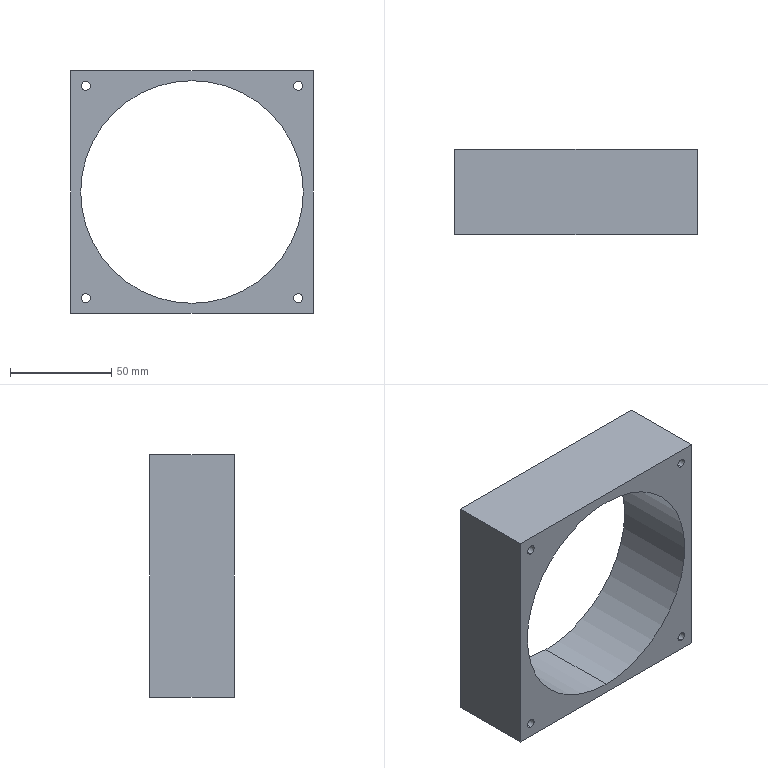Part | SolidWorks | features Extrusion 1, ICE 1 | 1 solid | 16 faces | box 120 x 42 x 120 mm | volume 202989 mm3 | cylinder 10 | plane 6 | commonest cylinder face diameters 4.5 x8 110 x2
STEP:
#1=CARTESIAN_POINT('',(-52.5,-21.,50.25));
#2=VERTEX_POINT('',#1);
#3=CARTESIAN_POINT('',(-52.5,-21.,54.75));
#4=VERTEX_POINT('',#3);
#5=CARTESIAN_POINT('',(-52.5,-21.,52.5));
#6=DIRECTION('',(0.,1.,0.));
#7=DIRECTION('',(0.,0.,-1.));
#8=AXIS2_PLACEMENT_3D('',#5,#6,#7);
#9=CIRCLE('',#8,2.25);
#10=EDGE_CURVE('',#2,#4,#9,.T.);
#11=ORIENTED_EDGE('',*,*,#10,.F.);
#12=CARTESIAN_POINT('',(-52.5,21.,50.25));
#13=VERTEX_POINT('',#12);
#14=CARTESIAN_POINT('',(-52.5,-21.,50.25));
#15=DIRECTION('',(0.,1.,0.));
#16=VECTOR('',#15,1000.);
#17=LINE('',#14,#16);
#18=EDGE_CURVE('',#2,#13,#17,.T.);
#19=ORIENTED_EDGE('',*,*,#18,.T.);
#20=CARTESIAN_POINT('',(-52.5,21.,54.75));
#21=VERTEX_POINT('',#20);
#22=CARTESIAN_POINT('',(-52.5,21.,52.5));
#23=DIRECTION('',(0.,1.,0.));
#24=DIRECTION('',(0.,0.,1.));
#25=AXIS2_PLACEMENT_3D('',#22,#23,#24);
#26=CIRCLE('',#25,2.25);
#27=EDGE_CURVE('',#13,#21,#26,.T.);
#28=ORIENTED_EDGE('',*,*,#27,.T.);
#29=CARTESIAN_POINT('',(-52.5,-21.,54.75));
#30=DIRECTION('',(0.,1.,0.));
#31=VECTOR('',#30,1000.);
#32=LINE('',#29,#31);
#33=EDGE_CURVE('',#4,#21,#32,.T.);
#34=ORIENTED_EDGE('',*,*,#33,.F.);
#35=EDGE_LOOP('',(#11,#19,#28,#34));
#36=FACE_OUTER_BOUND('',#35,.T.);
#37=CARTESIAN_POINT('',(-52.5,-21.,52.5));
#38=DIRECTION('',(0.,1.,0.));
#39=DIRECTION('',(0.,0.,1.));
#40=AXIS2_PLACEMENT_3D('',#37,#38,#39);
#41=CYLINDRICAL_SURFACE('',#40,2.25);
#42=ADVANCED_FACE('',(#36),#41,.F.);
#43=CARTESIAN_POINT('',(52.5,-21.,50.25));
#44=VERTEX_POINT('',#43);
#45=CARTESIAN_POINT('',(52.5,-21.,54.75));
#46=VERTEX_POINT('',#45);
#47=CARTESIAN_POINT('',(52.5,-21.,52.5));
#48=DIRECTION('',(0.,1.,0.));
#49=DIRECTION('',(0.,0.,1.));
#50=AXIS2_PLACEMENT_3D('',#47,#48,#49);
#51=CIRCLE('',#50,2.25);
#52=EDGE_CURVE('',#44,#46,#51,.T.);
#53=ORIENTED_EDGE('',*,*,#52,.F.);
#54=CARTESIAN_POINT('',(52.5,21.,50.25));
#55=VERTEX_POINT('',#54);
#56=CARTESIAN_POINT('',(52.5,-21.,50.25));
#57=DIRECTION('',(0.,1.,0.));
#58=VECTOR('',#57,1000.);
#59=LINE('',#56,#58);
#60=EDGE_CURVE('',#44,#55,#59,.T.);
#61=ORIENTED_EDGE('',*,*,#60,.T.);
#62=CARTESIAN_POINT('',(52.5,21.,54.75));
#63=VERTEX_POINT('',#62);
#64=CARTESIAN_POINT('',(52.5,21.,52.5));
#65=DIRECTION('',(0.,1.,0.));
#66=DIRECTION('',(0.,0.,1.));
#67=AXIS2_PLACEMENT_3D('',#64,#65,#66);
#68=CIRCLE('',#67,2.25);
#69=EDGE_CURVE('',#55,#63,#68,.T.);
#70=ORIENTED_EDGE('',*,*,#69,.T.);
#71=CARTESIAN_POINT('',(52.5,-21.,54.75));
#72=DIRECTION('',(0.,1.,0.));
#73=VECTOR('',#72,1000.);
#74=LINE('',#71,#73);
#75=EDGE_CURVE('',#46,#63,#74,.T.);
#76=ORIENTED_EDGE('',*,*,#75,.F.);
#77=EDGE_LOOP('',(#53,#61,#70,#76));
#78=FACE_OUTER_BOUND('',#77,.T.);
#79=CARTESIAN_POINT('',(52.5,-21.,52.5));
#80=DIRECTION('',(0.,1.,0.));
#81=DIRECTION('',(0.,0.,1.));
#82=AXIS2_PLACEMENT_3D('',#79,#80,#81);
#83=CYLINDRICAL_SURFACE('',#82,2.25);
#84=ADVANCED_FACE('',(#78),#83,.F.);
#85=CARTESIAN_POINT('',(52.5,-21.,-54.75));
#86=VERTEX_POINT('',#85);
#87=CARTESIAN_POINT('',(52.5,-21.,-50.25));
#88=VERTEX_POINT('',#87);
#89=CARTESIAN_POINT('',(52.5,-21.,-52.5));
#90=DIRECTION('',(0.,1.,0.));
#91=DIRECTION('',(0.,0.,-1.));
#92=AXIS2_PLACEMENT_3D('',#89,#90,#91);
#93=CIRCLE('',#92,2.25);
#94=EDGE_CURVE('',#86,#88,#93,.T.);
#95=ORIENTED_EDGE('',*,*,#94,.F.);
#96=CARTESIAN_POINT('',(52.5,21.,-54.75));
#97=VERTEX_POINT('',#96);
#98=CARTESIAN_POINT('',(52.5,-21.,-54.75));
#99=DIRECTION('',(0.,1.,0.));
#100=VECTOR('',#99,1000.);
#101=LINE('',#98,#100);
#102=EDGE_CURVE('',#86,#97,#101,.T.);
#103=ORIENTED_EDGE('',*,*,#102,.T.);
#104=CARTESIAN_POINT('',(52.5,21.,-50.25));
#105=VERTEX_POINT('',#104);
#106=CARTESIAN_POINT('',(52.5,21.,-52.5));
#107=DIRECTION('',(0.,1.,0.));
#108=DIRECTION('',(0.,0.,1.));
#109=AXIS2_PLACEMENT_3D('',#106,#107,#108);
#110=CIRCLE('',#109,2.25);
#111=EDGE_CURVE('',#97,#105,#110,.T.);
#112=ORIENTED_EDGE('',*,*,#111,.T.);
#113=CARTESIAN_POINT('',(52.5,-21.,-50.25));
#114=DIRECTION('',(0.,1.,0.));
#115=VECTOR('',#114,1000.);
#116=LINE('',#113,#115);
#117=EDGE_CURVE('',#88,#105,#116,.T.);
#118=ORIENTED_EDGE('',*,*,#117,.F.);
#119=EDGE_LOOP('',(#95,#103,#112,#118));
#120=FACE_OUTER_BOUND('',#119,.T.);
#121=CARTESIAN_POINT('',(52.5,-21.,-52.5));
#122=DIRECTION('',(0.,1.,0.));
#123=DIRECTION('',(0.,0.,1.));
#124=AXIS2_PLACEMENT_3D('',#121,#122,#123);
#125=CYLINDRICAL_SURFACE('',#124,2.25);
#126=ADVANCED_FACE('',(#120),#125,.F.);
#127=CARTESIAN_POINT('',(-52.5,-21.,-54.75));
#128=VERTEX_POINT('',#127);
#129=CARTESIAN_POINT('',(-52.5,-21.,-50.25));
#130=VERTEX_POINT('',#129);
#131=CARTESIAN_POINT('',(-52.5,-21.,-52.5));
#132=DIRECTION('',(0.,1.,0.));
#133=DIRECTION('',(0.,0.,1.));
#134=AXIS2_PLACEMENT_3D('',#131,#132,#133);
#135=CIRCLE('',#134,2.25);
#136=EDGE_CURVE('',#128,#130,#135,.T.);
#137=ORIENTED_EDGE('',*,*,#136,.F.);
#138=CARTESIAN_POINT('',(-52.5,21.,-54.75));
#139=VERTEX_POINT('',#138);
#140=CARTESIAN_POINT('',(-52.5,-21.,-54.75));
#141=DIRECTION('',(0.,1.,0.));
#142=VECTOR('',#141,1000.);
#143=LINE('',#140,#142);
#144=EDGE_CURVE('',#128,#139,#143,.T.);
#145=ORIENTED_EDGE('',*,*,#144,.T.);
#146=CARTESIAN_POINT('',(-52.5,21.,-50.25));
#147=VERTEX_POINT('',#146);
#148=CARTESIAN_POINT('',(-52.5,21.,-52.5));
#149=DIRECTION('',(0.,1.,0.));
#150=DIRECTION('',(0.,0.,1.));
#151=AXIS2_PLACEMENT_3D('',#148,#149,#150);
#152=CIRCLE('',#151,2.25);
#153=EDGE_CURVE('',#139,#147,#152,.T.);
#154=ORIENTED_EDGE('',*,*,#153,.T.);
#155=CARTESIAN_POINT('',(-52.5,-21.,-50.25));
#156=DIRECTION('',(0.,1.,0.));
#157=VECTOR('',#156,1000.);
#158=LINE('',#155,#157);
#159=EDGE_CURVE('',#130,#147,#158,.T.);
#160=ORIENTED_EDGE('',*,*,#159,.F.);
#161=EDGE_LOOP('',(#137,#145,#154,#160));
#162=FACE_OUTER_BOUND('',#161,.T.);
#163=CARTESIAN_POINT('',(-52.5,-21.,-52.5));
#164=DIRECTION('',(0.,1.,0.));
#165=DIRECTION('',(0.,0.,1.));
#166=AXIS2_PLACEMENT_3D('',#163,#164,#165);
#167=CYLINDRICAL_SURFACE('',#166,2.25);
#168=ADVANCED_FACE('',(#162),#167,.F.);
#169=CARTESIAN_POINT('',(0.,-21.,-55.));
#170=VERTEX_POINT('',#169);
#171=CARTESIAN_POINT('',(0.,-21.,55.));
#172=VERTEX_POINT('',#171);
#173=CARTESIAN_POINT('',(0.,-21.,0.));
#174=DIRECTION('',(0.,1.,0.));
#175=DIRECTION('',(0.,0.,1.));
#176=AXIS2_PLACEMENT_3D('',#173,#174,#175);
#177=CIRCLE('',#176,55.);
#178=EDGE_CURVE('',#170,#172,#177,.T.);
#179=ORIENTED_EDGE('',*,*,#178,.F.);
#180=CARTESIAN_POINT('',(0.,21.,-55.));
#181=VERTEX_POINT('',#180);
#182=CARTESIAN_POINT('',(0.,-21.,-55.));
#183=DIRECTION('',(0.,1.,0.));
#184=VECTOR('',#183,1000.);
#185=LINE('',#182,#184);
#186=EDGE_CURVE('',#170,#181,#185,.T.);
#187=ORIENTED_EDGE('',*,*,#186,.T.);
#188=CARTESIAN_POINT('',(0.,21.,55.));
#189=VERTEX_POINT('',#188);
#190=CARTESIAN_POINT('',(0.,21.,0.));
#191=DIRECTION('',(0.,1.,0.));
#192=DIRECTION('',(0.,0.,1.));
#193=AXIS2_PLACEMENT_3D('',#190,#191,#192);
#194=CIRCLE('',#193,55.);
#195=EDGE_CURVE('',#181,#189,#194,.T.);
#196=ORIENTED_EDGE('',*,*,#195,.T.);
#197=CARTESIAN_POINT('',(0.,-21.,55.));
#198=DIRECTION('',(0.,1.,0.));
#199=VECTOR('',#198,1000.);
#200=LINE('',#197,#199);
#201=EDGE_CURVE('',#172,#189,#200,.T.);
#202=ORIENTED_EDGE('',*,*,#201,.F.);
#203=EDGE_LOOP('',(#179,#187,#196,#202));
#204=FACE_OUTER_BOUND('',#203,.T.);
#205=CARTESIAN_POINT('',(0.,-21.,0.));
#206=DIRECTION('',(0.,1.,0.));
#207=DIRECTION('',(0.,0.,1.));
#208=AXIS2_PLACEMENT_3D('',#205,#206,#207);
#209=CYLINDRICAL_SURFACE('',#208,55.);
#210=ADVANCED_FACE('',(#204),#209,.F.);
#211=CARTESIAN_POINT('',(60.,-21.,60.));
#212=VERTEX_POINT('',#211);
#213=CARTESIAN_POINT('',(60.,-21.,-60.));
#214=VERTEX_POINT('',#213);
#215=CARTESIAN_POINT('',(60.,-21.,-60.));
#216=DIRECTION('',(0.,0.,-1.));
#217=VECTOR('',#216,1000.);
#218=LINE('',#215,#217);
#219=EDGE_CURVE('',#212,#214,#218,.T.);
#220=ORIENTED_EDGE('',*,*,#219,.T.);
#221=CARTESIAN_POINT('',(60.,21.,-60.));
#222=VERTEX_POINT('',#221);
#223=CARTESIAN_POINT('',(60.,21.,-60.));
#224=DIRECTION('',(0.,-1.,0.));
#225=VECTOR('',#224,1000.);
#226=LINE('',#223,#225);
#227=EDGE_CURVE('',#222,#214,#226,.T.);
#228=ORIENTED_EDGE('',*,*,#227,.F.);
#229=CARTESIAN_POINT('',(60.,21.,60.));
#230=VERTEX_POINT('',#229);
#231=CARTESIAN_POINT('',(60.,21.,-60.));
#232=DIRECTION('',(0.,0.,-1.));
#233=VECTOR('',#232,1000.);
#234=LINE('',#231,#233);
#235=EDGE_CURVE('',#230,#222,#234,.T.);
#236=ORIENTED_EDGE('',*,*,#235,.F.);
#237=CARTESIAN_POINT('',(60.,21.,60.));
#238=DIRECTION('',(0.,-1.,0.));
#239=VECTOR('',#238,1000.);
#240=LINE('',#237,#239);
#241=EDGE_CURVE('',#230,#212,#240,.T.);
#242=ORIENTED_EDGE('',*,*,#241,.T.);
#243=EDGE_LOOP('',(#220,#228,#236,#242));
#244=FACE_OUTER_BOUND('',#243,.T.);
#245=CARTESIAN_POINT('',(60.,21.,-60.));
#246=DIRECTION('',(-1.,0.,0.));
#247=DIRECTION('',(0.,0.,1.));
#248=AXIS2_PLACEMENT_3D('',#245,#246,#247);
#249=PLANE('',#248);
#250=ADVANCED_FACE('',(#244),#249,.F.);
#251=CARTESIAN_POINT('',(-60.,-21.,-60.));
#252=VERTEX_POINT('',#251);
#253=CARTESIAN_POINT('',(-60.,-21.,-60.));
#254=DIRECTION('',(-1.,0.,0.));
#255=VECTOR('',#254,1000.);
#256=LINE('',#253,#255);
#257=EDGE_CURVE('',#214,#252,#256,.T.);
#258=ORIENTED_EDGE('',*,*,#257,.T.);
#259=CARTESIAN_POINT('',(-60.,21.,-60.));
#260=VERTEX_POINT('',#259);
#261=CARTESIAN_POINT('',(-60.,21.,-60.));
#262=DIRECTION('',(0.,-1.,0.));
#263=VECTOR('',#262,1000.);
#264=LINE('',#261,#263);
#265=EDGE_CURVE('',#260,#252,#264,.T.);
#266=ORIENTED_EDGE('',*,*,#265,.F.);
#267=CARTESIAN_POINT('',(-60.,21.,-60.));
#268=DIRECTION('',(-1.,0.,0.));
#269=VECTOR('',#268,1000.);
#270=LINE('',#267,#269);
#271=EDGE_CURVE('',#222,#260,#270,.T.);
#272=ORIENTED_EDGE('',*,*,#271,.F.);
#273=ORIENTED_EDGE('',*,*,#227,.T.);
#274=EDGE_LOOP('',(#258,#266,#272,#273));
#275=FACE_OUTER_BOUND('',#274,.T.);
#276=CARTESIAN_POINT('',(-60.,21.,-60.));
#277=DIRECTION('',(0.,0.,1.));
#278=DIRECTION('',(1.,0.,0.));
#279=AXIS2_PLACEMENT_3D('',#276,#277,#278);
#280=PLANE('',#279);
#281=ADVANCED_FACE('',(#275),#280,.F.);
#282=CARTESIAN_POINT('',(-60.,-21.,60.));
#283=VERTEX_POINT('',#282);
#284=CARTESIAN_POINT('',(-60.,-21.,-60.));
#285=DIRECTION('',(0.,0.,1.));
#286=VECTOR('',#285,1000.);
#287=LINE('',#284,#286);
#288=EDGE_CURVE('',#252,#283,#287,.T.);
#289=ORIENTED_EDGE('',*,*,#288,.T.);
#290=CARTESIAN_POINT('',(-60.,21.,60.));
#291=VERTEX_POINT('',#290);
#292=CARTESIAN_POINT('',(-60.,21.,60.));
#293=DIRECTION('',(0.,-1.,0.));
#294=VECTOR('',#293,1000.);
#295=LINE('',#292,#294);
#296=EDGE_CURVE('',#291,#283,#295,.T.);
#297=ORIENTED_EDGE('',*,*,#296,.F.);
#298=CARTESIAN_POINT('',(-60.,21.,-60.));
#299=DIRECTION('',(0.,0.,1.));
#300=VECTOR('',#299,1000.);
#301=LINE('',#298,#300);
#302=EDGE_CURVE('',#260,#291,#301,.T.);
#303=ORIENTED_EDGE('',*,*,#302,.F.);
#304=ORIENTED_EDGE('',*,*,#265,.T.);
#305=EDGE_LOOP('',(#289,#297,#303,#304));
#306=FACE_OUTER_BOUND('',#305,.T.);
#307=CARTESIAN_POINT('',(-60.,21.,-60.));
#308=DIRECTION('',(1.,0.,0.));
#309=DIRECTION('',(0.,0.,-1.));
#310=AXIS2_PLACEMENT_3D('',#307,#308,#309);
#311=PLANE('',#310);
#312=ADVANCED_FACE('',(#306),#311,.F.);
#313=CARTESIAN_POINT('',(-60.,-21.,60.));
#314=DIRECTION('',(1.,0.,0.));
#315=VECTOR('',#314,1000.);
#316=LINE('',#313,#315);
#317=EDGE_CURVE('',#283,#212,#316,.T.);
#318=ORIENTED_EDGE('',*,*,#317,.T.);
#319=ORIENTED_EDGE('',*,*,#241,.F.);
#320=CARTESIAN_POINT('',(-60.,21.,60.));
#321=DIRECTION('',(1.,0.,0.));
#322=VECTOR('',#321,1000.);
#323=LINE('',#320,#322);
#324=EDGE_CURVE('',#291,#230,#323,.T.);
#325=ORIENTED_EDGE('',*,*,#324,.F.);
#326=ORIENTED_EDGE('',*,*,#296,.T.);
#327=EDGE_LOOP('',(#318,#319,#325,#326));
#328=FACE_OUTER_BOUND('',#327,.T.);
#329=CARTESIAN_POINT('',(-60.,21.,60.));
#330=DIRECTION('',(0.,0.,-1.));
#331=DIRECTION('',(-1.,0.,0.));
#332=AXIS2_PLACEMENT_3D('',#329,#330,#331);
#333=PLANE('',#332);
#334=ADVANCED_FACE('',(#328),#333,.F.);
#335=CARTESIAN_POINT('',(-52.5,21.,52.5));
#336=DIRECTION('',(0.,1.,0.));
#337=DIRECTION('',(0.,0.,1.));
#338=AXIS2_PLACEMENT_3D('',#335,#336,#337);
#339=CIRCLE('',#338,2.25);
#340=EDGE_CURVE('',#21,#13,#339,.T.);
#341=ORIENTED_EDGE('',*,*,#340,.F.);
#342=ORIENTED_EDGE('',*,*,#27,.F.);
#343=EDGE_LOOP('',(#341,#342));
#344=FACE_BOUND('',#343,.T.);
#345=CARTESIAN_POINT('',(52.5,21.,52.5));
#346=DIRECTION('',(0.,1.,0.));
#347=DIRECTION('',(0.,0.,1.));
#348=AXIS2_PLACEMENT_3D('',#345,#346,#347);
#349=CIRCLE('',#348,2.25);
#350=EDGE_CURVE('',#63,#55,#349,.T.);
#351=ORIENTED_EDGE('',*,*,#350,.F.);
#352=ORIENTED_EDGE('',*,*,#69,.F.);
#353=EDGE_LOOP('',(#351,#352));
#354=FACE_BOUND('',#353,.T.);
#355=CARTESIAN_POINT('',(52.5,21.,-52.5));
#356=DIRECTION('',(0.,1.,0.));
#357=DIRECTION('',(0.,0.,1.));
#358=AXIS2_PLACEMENT_3D('',#355,#356,#357);
#359=CIRCLE('',#358,2.25);
#360=EDGE_CURVE('',#105,#97,#359,.T.);
#361=ORIENTED_EDGE('',*,*,#360,.F.);
#362=ORIENTED_EDGE('',*,*,#111,.F.);
#363=EDGE_LOOP('',(#361,#362));
#364=FACE_BOUND('',#363,.T.);
#365=CARTESIAN_POINT('',(-52.5,21.,-52.5));
#366=DIRECTION('',(0.,1.,0.));
#367=DIRECTION('',(0.,0.,1.));
#368=AXIS2_PLACEMENT_3D('',#365,#366,#367);
#369=CIRCLE('',#368,2.25);
#370=EDGE_CURVE('',#147,#139,#369,.T.);
#371=ORIENTED_EDGE('',*,*,#370,.F.);
#372=ORIENTED_EDGE('',*,*,#153,.F.);
#373=EDGE_LOOP('',(#371,#372));
#374=FACE_BOUND('',#373,.T.);
#375=CARTESIAN_POINT('',(0.,21.,0.));
#376=DIRECTION('',(0.,1.,0.));
#377=DIRECTION('',(0.,0.,1.));
#378=AXIS2_PLACEMENT_3D('',#375,#376,#377);
#379=CIRCLE('',#378,55.);
#380=EDGE_CURVE('',#189,#181,#379,.T.);
#381=ORIENTED_EDGE('',*,*,#380,.F.);
#382=ORIENTED_EDGE('',*,*,#195,.F.);
#383=EDGE_LOOP('',(#381,#382));
#384=FACE_BOUND('',#383,.T.);
#385=ORIENTED_EDGE('',*,*,#235,.T.);
#386=ORIENTED_EDGE('',*,*,#271,.T.);
#387=ORIENTED_EDGE('',*,*,#302,.T.);
#388=ORIENTED_EDGE('',*,*,#324,.T.);
#389=EDGE_LOOP('',(#385,#386,#387,#388));
#390=FACE_OUTER_BOUND('',#389,.T.);
#391=CARTESIAN_POINT('',(0.,21.,0.));
#392=DIRECTION('',(0.,1.,0.));
#393=DIRECTION('',(0.,0.,1.));
#394=AXIS2_PLACEMENT_3D('',#391,#392,#393);
#395=PLANE('',#394);
#396=ADVANCED_FACE('',(#344,#354,#364,#374,#384,#390),#395,.T.);
#397=CARTESIAN_POINT('',(-52.5,-21.,52.5));
#398=DIRECTION('',(0.,1.,0.));
#399=DIRECTION('',(0.,0.,-1.));
#400=AXIS2_PLACEMENT_3D('',#397,#398,#399);
#401=CIRCLE('',#400,2.25);
#402=EDGE_CURVE('',#4,#2,#401,.T.);
#403=ORIENTED_EDGE('',*,*,#402,.T.);
#404=ORIENTED_EDGE('',*,*,#10,.T.);
#405=EDGE_LOOP('',(#403,#404));
#406=FACE_BOUND('',#405,.T.);
#407=CARTESIAN_POINT('',(52.5,-21.,52.5));
#408=DIRECTION('',(0.,1.,0.));
#409=DIRECTION('',(0.,0.,1.));
#410=AXIS2_PLACEMENT_3D('',#407,#408,#409);
#411=CIRCLE('',#410,2.25);
#412=EDGE_CURVE('',#46,#44,#411,.T.);
#413=ORIENTED_EDGE('',*,*,#412,.T.);
#414=ORIENTED_EDGE('',*,*,#52,.T.);
#415=EDGE_LOOP('',(#413,#414));
#416=FACE_BOUND('',#415,.T.);
#417=CARTESIAN_POINT('',(52.5,-21.,-52.5));
#418=DIRECTION('',(0.,1.,0.));
#419=DIRECTION('',(0.,0.,-1.));
#420=AXIS2_PLACEMENT_3D('',#417,#418,#419);
#421=CIRCLE('',#420,2.25);
#422=EDGE_CURVE('',#88,#86,#421,.T.);
#423=ORIENTED_EDGE('',*,*,#422,.T.);
#424=ORIENTED_EDGE('',*,*,#94,.T.);
#425=EDGE_LOOP('',(#423,#424));
#426=FACE_BOUND('',#425,.T.);
#427=CARTESIAN_POINT('',(-52.5,-21.,-52.5));
#428=DIRECTION('',(0.,1.,0.));
#429=DIRECTION('',(0.,0.,1.));
#430=AXIS2_PLACEMENT_3D('',#427,#428,#429);
#431=CIRCLE('',#430,2.25);
#432=EDGE_CURVE('',#130,#128,#431,.T.);
#433=ORIENTED_EDGE('',*,*,#432,.T.);
#434=ORIENTED_EDGE('',*,*,#136,.T.);
#435=EDGE_LOOP('',(#433,#434));
#436=FACE_BOUND('',#435,.T.);
#437=CARTESIAN_POINT('',(0.,-21.,0.));
#438=DIRECTION('',(0.,1.,0.));
#439=DIRECTION('',(0.,0.,1.));
#440=AXIS2_PLACEMENT_3D('',#437,#438,#439);
#441=CIRCLE('',#440,55.);
#442=EDGE_CURVE('',#172,#170,#441,.T.);
#443=ORIENTED_EDGE('',*,*,#442,.T.);
#444=ORIENTED_EDGE('',*,*,#178,.T.);
#445=EDGE_LOOP('',(#443,#444));
#446=FACE_BOUND('',#445,.T.);
#447=ORIENTED_EDGE('',*,*,#219,.F.);
#448=ORIENTED_EDGE('',*,*,#317,.F.);
#449=ORIENTED_EDGE('',*,*,#288,.F.);
#450=ORIENTED_EDGE('',*,*,#257,.F.);
#451=EDGE_LOOP('',(#447,#448,#449,#450));
#452=FACE_OUTER_BOUND('',#451,.T.);
#453=CARTESIAN_POINT('',(0.,-21.,0.));
#454=DIRECTION('',(0.,1.,0.));
#455=DIRECTION('',(0.,0.,1.));
#456=AXIS2_PLACEMENT_3D('',#453,#454,#455);
#457=PLANE('',#456);
#458=ADVANCED_FACE('',(#406,#416,#426,#436,#446,#452),#457,.F.);
#459=ORIENTED_EDGE('',*,*,#186,.F.);
#460=ORIENTED_EDGE('',*,*,#442,.F.);
#461=ORIENTED_EDGE('',*,*,#201,.T.);
#462=ORIENTED_EDGE('',*,*,#380,.T.);
#463=EDGE_LOOP('',(#459,#460,#461,#462));
#464=FACE_OUTER_BOUND('',#463,.T.);
#465=CARTESIAN_POINT('',(0.,-21.,0.));
#466=DIRECTION('',(0.,1.,0.));
#467=DIRECTION('',(0.,0.,1.));
#468=AXIS2_PLACEMENT_3D('',#465,#466,#467);
#469=CYLINDRICAL_SURFACE('',#468,55.);
#470=ADVANCED_FACE('',(#464),#469,.F.);
#471=ORIENTED_EDGE('',*,*,#144,.F.);
#472=ORIENTED_EDGE('',*,*,#432,.F.);
#473=ORIENTED_EDGE('',*,*,#159,.T.);
#474=ORIENTED_EDGE('',*,*,#370,.T.);
#475=EDGE_LOOP('',(#471,#472,#473,#474));
#476=FACE_OUTER_BOUND('',#475,.T.);
#477=CARTESIAN_POINT('',(-52.5,-21.,-52.5));
#478=DIRECTION('',(0.,1.,0.));
#479=DIRECTION('',(0.,0.,1.));
#480=AXIS2_PLACEMENT_3D('',#477,#478,#479);
#481=CYLINDRICAL_SURFACE('',#480,2.25);
#482=ADVANCED_FACE('',(#476),#481,.F.);
#483=ORIENTED_EDGE('',*,*,#102,.F.);
#484=ORIENTED_EDGE('',*,*,#422,.F.);
#485=ORIENTED_EDGE('',*,*,#117,.T.);
#486=ORIENTED_EDGE('',*,*,#360,.T.);
#487=EDGE_LOOP('',(#483,#484,#485,#486));
#488=FACE_OUTER_BOUND('',#487,.T.);
#489=CARTESIAN_POINT('',(52.5,-21.,-52.5));
#490=DIRECTION('',(0.,1.,0.));
#491=DIRECTION('',(0.,0.,1.));
#492=AXIS2_PLACEMENT_3D('',#489,#490,#491);
#493=CYLINDRICAL_SURFACE('',#492,2.25);
#494=ADVANCED_FACE('',(#488),#493,.F.);
#495=ORIENTED_EDGE('',*,*,#60,.F.);
#496=ORIENTED_EDGE('',*,*,#412,.F.);
#497=ORIENTED_EDGE('',*,*,#75,.T.);
#498=ORIENTED_EDGE('',*,*,#350,.T.);
#499=EDGE_LOOP('',(#495,#496,#497,#498));
#500=FACE_OUTER_BOUND('',#499,.T.);
#501=CARTESIAN_POINT('',(52.5,-21.,52.5));
#502=DIRECTION('',(0.,1.,0.));
#503=DIRECTION('',(0.,0.,1.));
#504=AXIS2_PLACEMENT_3D('',#501,#502,#503);
#505=CYLINDRICAL_SURFACE('',#504,2.25);
#506=ADVANCED_FACE('',(#500),#505,.F.);
#507=ORIENTED_EDGE('',*,*,#18,.F.);
#508=ORIENTED_EDGE('',*,*,#402,.F.);
#509=ORIENTED_EDGE('',*,*,#33,.T.);
#510=ORIENTED_EDGE('',*,*,#340,.T.);
#511=EDGE_LOOP('',(#507,#508,#509,#510));
#512=FACE_OUTER_BOUND('',#511,.T.);
#513=CARTESIAN_POINT('',(-52.5,-21.,52.5));
#514=DIRECTION('',(0.,1.,0.));
#515=DIRECTION('',(0.,0.,1.));
#516=AXIS2_PLACEMENT_3D('',#513,#514,#515);
#517=CYLINDRICAL_SURFACE('',#516,2.25);
#518=ADVANCED_FACE('',(#512),#517,.F.);
#519=CLOSED_SHELL('',(#42,#84,#126,#168,#210,#250,#281,#312,#334,#396,#458,#470,#482,#494,#506,#518));
#520=MANIFOLD_SOLID_BREP('',#519);
#521=CARTESIAN_POINT('',(0.,0.,0.));
#522=DIRECTION('',(0.,0.,1.));
#523=DIRECTION('',(1.,0.,0.));
#524=AXIS2_PLACEMENT_3D('',#521,#522,#523);
#525=(LENGTH_UNIT()NAMED_UNIT(*)SI_UNIT(.MILLI.,.METRE.));
#526=UNCERTAINTY_MEASURE_WITH_UNIT(LENGTH_MEASURE(0.00001),#525,'','');
#527=(NAMED_UNIT(*)PLANE_ANGLE_UNIT()SI_UNIT($,.RADIAN.));
#528=(NAMED_UNIT(*)SI_UNIT($,.STERADIAN.)SOLID_ANGLE_UNIT());
#529=(GEOMETRIC_REPRESENTATION_CONTEXT(3)GLOBAL_UNCERTAINTY_ASSIGNED_CONTEXT((#526))GLOBAL_UNIT_ASSIGNED_CONTEXT((#525,#527,#528))REPRESENTATION_CONTEXT('',''));
#530=ADVANCED_BREP_SHAPE_REPRESENTATION('',(#520,#524),#529);